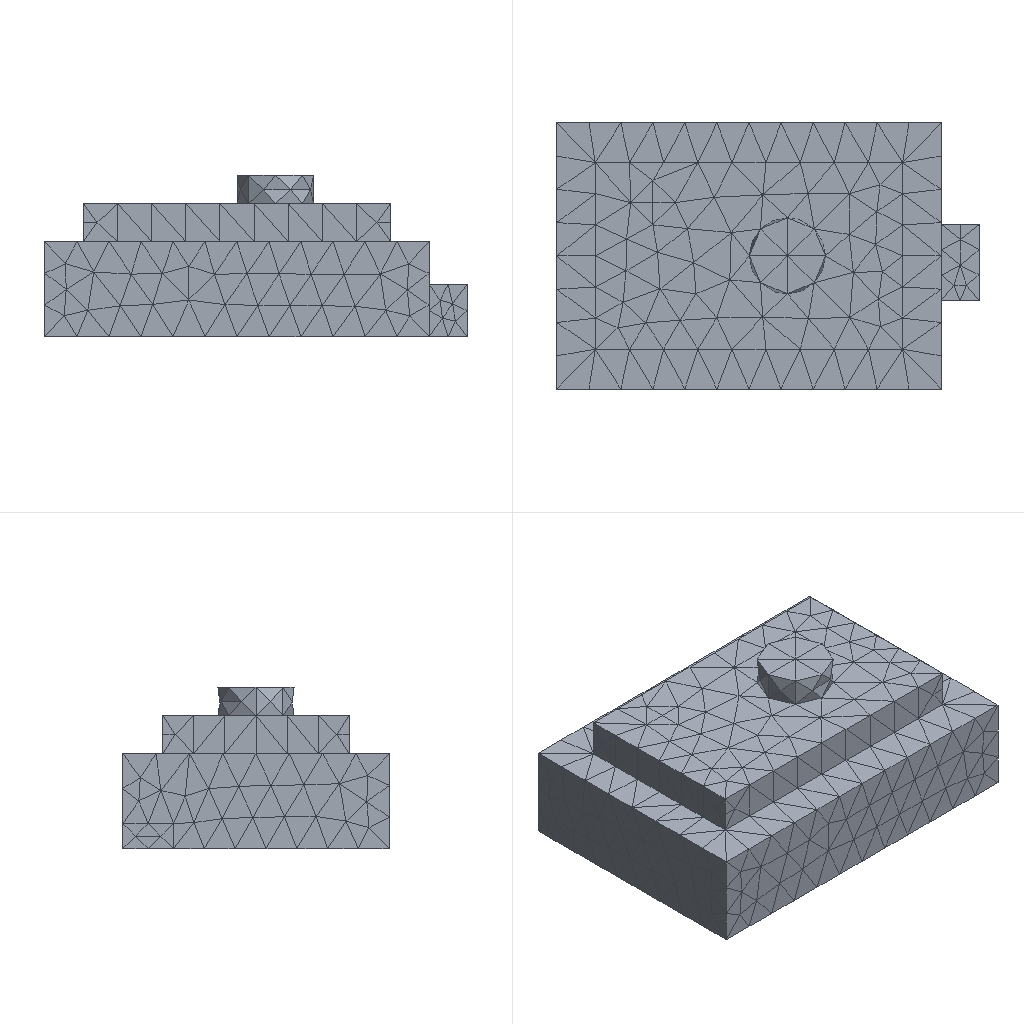Simulation study | ansys mapdl
Set-up summary:
category,name,step,type,value,unit,region
solver,ansys_mapdl
units,mm-N-s-tonne (MPa),,inferred,E=210000 density=
analysis,model,,static
mesh,nodes,,,4905
mesh,elements,,,2929
element_type,SOLID187,,,2929
material,mat 1,,E,210000
material,mat 1,,nu,0.3
load,,model,body load temp,,,all
load,,model,force,"1000 [dir=(0, 0, -1) n=342]",,node list
bc,,model,fixed,"[dofs=UX,UY,UZ n=5838]",,node list
Ansys APDL input file, long lists of numbers shortened:
/COM,ANSYS RELEASE 2026 R1           BUILD 26.1      UP20260202       09:08:11
/PREP7
/NOPR
/TITLE,2
ANTYPE, 0
*IF,_CDRDOFF,EQ,1,THEN     !if solid model was read in
_CDRDOFF=             !reset flag, numoffs already performed
*ELSE              !offset database for the following FE model
NUMOFF,NODE,     4905
NUMOFF,ELEM,     2929
NUMOFF,MAT ,        1
NUMOFF,TYPE,        1
*ENDIF
*SET,_RETURN ,  0.
*SET,_STATUS ,  0.
*SET,_UIQR   ,  342.
*SET,__FLOATPARAMETER__,  4905.
DOF,DELETE
ETBLOCK,        1,        1
(2i9,19a9)
        1      187        0        0        0        0        0        0        0        0        0        0        0        0        0        0        0        0        0        0        0
       -1
NBLOCK,6,SOLID,      4905,      4905
(3i9,6e21.13e3)
        1        0        0-4.4575000000000E+001 4.2000000000000E+001 8.0000000000000E+000
! (4904 more lines like these left out)
N,UNBL,LOC,       -1,
EBLOCK,19,SOLID,      2929,      2929
(19i10)
         1         1         1         1         0         0         0         0        10         0         1      1895      1896      1546      1897      2172      2173      2174      2175
! (5857 more lines like these left out)
        -1
MPTEMP,UNBL, 1, 1,  0.    ,
MPDATA,UNBL, 1,EX  ,       1, 1,  210000.000    ,
MPTEMP,UNBL, 1, 1,  0.    ,
MPDATA,UNBL, 1,NUXY,       1, 1, 0.3    ,
MPTEMP,UNBL, 1, 1,  0.    ,
MPDATA,UNBL, 1,PRXY,       1, 1, 0.3    ,
EXTOPT,ATTR,      0,      0,      0
EXTOPT,ESIZE,  0,  0.
EXTOPT,ACLEAR,      0
TREF,  0.
IRLF,  0
BFUNIF,TEMP,_TINY
ACEL,  0.    ,  0.    ,  0.
OMEGA,  0.    ,  0.    ,  0.
DOMEGA,  0.    ,  0.    ,  0.
CGLOC,  0.    ,  0.    ,  0.
CGOMEGA,  0.    ,  0.    ,  0.
DCGOMG,  0.    ,  0.    ,  0.
KUSE,     0
TIME,  0.
ALPHAD,  0.
BETAD,  0.
DMPRAT,  0.
DMPSTR,  0.
CRPLIM, 0.1    ,   0
CRPLIM,  0.    ,   1
NCNV,     0, 1.000000000E+12,     0,  0.    ,  0.
NEQIT,     0
ERESX,DEFA
DBLOCK,      5838
(i9,a6,2(pg16.9))
        1  UX    0.00000000      0.00000000
! (5837 more lines like these left out)
       -1
FBLOCK,       342
(i9,a6,2(pg16.9))
      556  FZ   -2.92397661      0.00000000
! (341 more lines like these left out)
       -1
/GO
FINISH
Results summary:
result,analysis_type_db,,,static,unstated
result,n_sets,,,1,unstated
result,load_steps[0].set,load_step=1,,1,unstated
result,load_steps[0].substep,load_step=1,,1,unstated
result,load_steps[0].time,load_step=1,,1,unstated
result,load_steps[0].freq,load_step=1,,1,unstated
result,load_steps[0].max_usum,load_step=1,,7.65254e-05,unstated
result,load_steps[0].max_seqv,load_step=1,,0.9162,unstated
result,load_steps[0].reaction_sum.FX,load_step=1,,-1.9164e-11,unstated
result,load_steps[0].reaction_sum.FY,load_step=1,,3.46745e-12,unstated
result,load_steps[0].reaction_sum.FZ,load_step=1,,1000,unstated
result,load_steps[0].reaction_sum.MX,load_step=1,,0,unstated
result,load_steps[0].reaction_sum.MY,load_step=1,,0,unstated
result,load_steps[0].reaction_sum.MZ,load_step=1,,0,unstated
result,convergence,,,results present for all listed sets,unstated